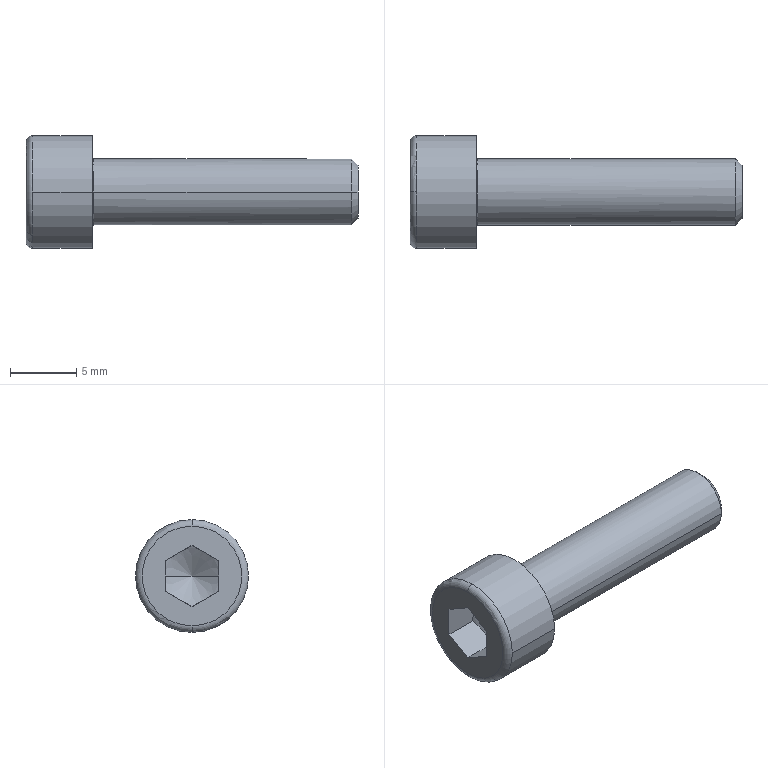Part | STEP file | KS B 1003 - M 5 x 20 | 1 solid | 21 faces | box 25 x 8.5 x 8.5 mm | volume 631.412 mm3 | plane 9 | torus 4 | cylinder 4 | cone 4 | commonest cylinder face diameters 5 x2 8.5 x2